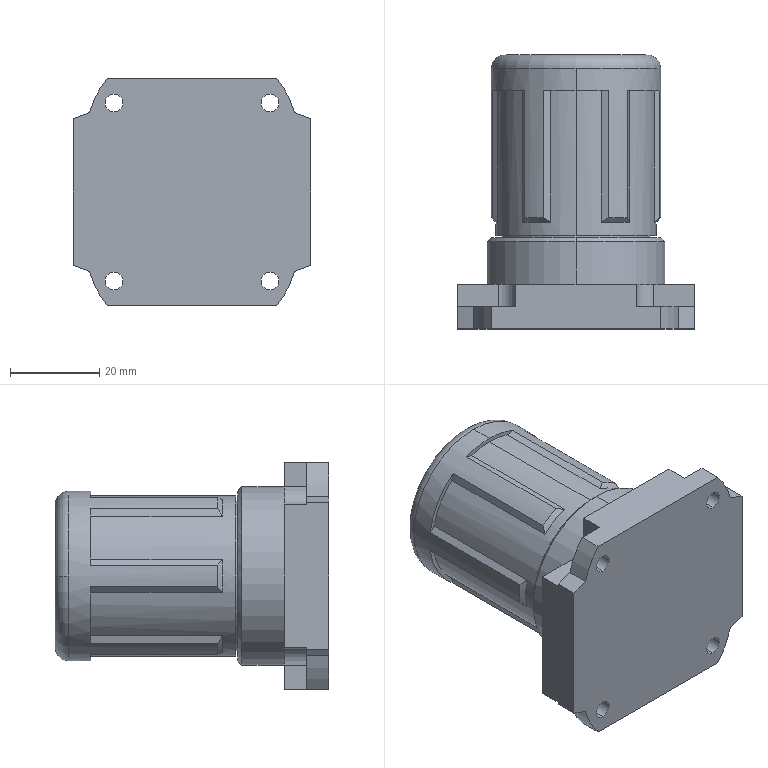Part | SolidWorks | features BaseBody 1 | 1 solid | 191 faces | box 53.4 x 61.5 x 51 mm | volume 80165 mm3 | plane 123 | cylinder 58 | cone 8 | torus 2 | commonest cylinder face diameters 4 x8 0.698 x6 40 x6 0.775 x5 0.465 x4 0.62 x4